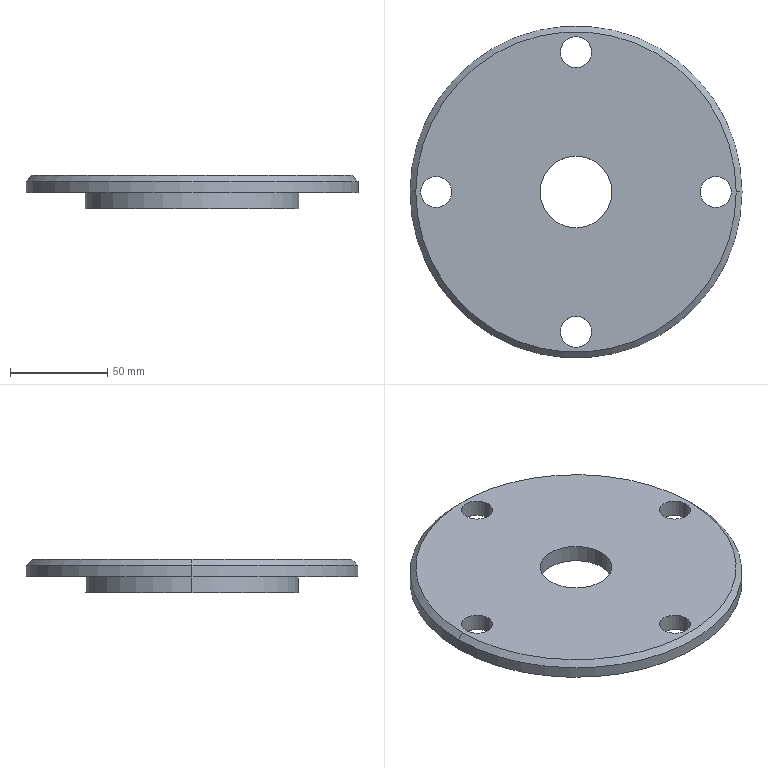Part | NX | features BREP 1 | 1 solid | 22 faces | box 171 x 171 x 17 mm | volume 205475 mm3 | cylinder 14 | cone 4 | plane 4 | commonest cylinder face diameters 16 x8 37 x2 110 x2 171 x2
STEP:
#1=CARTESIAN_POINT('',(-64.,0.,-9.));
#2=VERTEX_POINT('',#1);
#3=CARTESIAN_POINT('',(-80.,0.,-9.));
#4=VERTEX_POINT('',#3);
#5=CARTESIAN_POINT('',(-72.,0.,-9.));
#6=DIRECTION('',(0.,0.,-1.));
#7=DIRECTION('',(1.,0.,0.));
#8=AXIS2_PLACEMENT_3D('',#5,#6,#7);
#9=CIRCLE('',#8,8.);
#10=EDGE_CURVE('',#2,#4,#9,.T.);
#11=ORIENTED_EDGE('',*,*,#10,.T.);
#12=CARTESIAN_POINT('',(-80.,0.,0.));
#13=VERTEX_POINT('',#12);
#14=CARTESIAN_POINT('',(-80.,0.,-17.001));
#15=DIRECTION('',(0.,0.,1.));
#16=VECTOR('',#15,1000.);
#17=LINE('',#14,#16);
#18=EDGE_CURVE('',#4,#13,#17,.T.);
#19=ORIENTED_EDGE('',*,*,#18,.T.);
#20=CARTESIAN_POINT('',(-64.,0.,0.));
#21=VERTEX_POINT('',#20);
#22=CARTESIAN_POINT('',(-72.,0.,0.));
#23=DIRECTION('',(0.,0.,1.));
#24=DIRECTION('',(1.,0.,0.));
#25=AXIS2_PLACEMENT_3D('',#22,#23,#24);
#26=CIRCLE('',#25,8.);
#27=EDGE_CURVE('',#13,#21,#26,.T.);
#28=ORIENTED_EDGE('',*,*,#27,.T.);
#29=CARTESIAN_POINT('',(-64.,0.,-17.001));
#30=DIRECTION('',(0.,0.,1.));
#31=VECTOR('',#30,1000.);
#32=LINE('',#29,#31);
#33=EDGE_CURVE('',#2,#21,#32,.T.);
#34=ORIENTED_EDGE('',*,*,#33,.F.);
#35=EDGE_LOOP('',(#11,#19,#28,#34));
#36=FACE_BOUND('',#35,.T.);
#37=CARTESIAN_POINT('',(-72.,0.,-17.001));
#38=DIRECTION('',(0.,0.,1.));
#39=DIRECTION('',(-1.,0.,0.));
#40=AXIS2_PLACEMENT_3D('',#37,#38,#39);
#41=CYLINDRICAL_SURFACE('',#40,8.);
#42=ADVANCED_FACE('',(#36),#41,.F.);
#43=CARTESIAN_POINT('',(8.,-72.,-9.));
#44=VERTEX_POINT('',#43);
#45=CARTESIAN_POINT('',(-8.,-72.,-9.));
#46=VERTEX_POINT('',#45);
#47=CARTESIAN_POINT('',(0.,-72.,-9.));
#48=DIRECTION('',(0.,0.,-1.));
#49=DIRECTION('',(1.,0.,0.));
#50=AXIS2_PLACEMENT_3D('',#47,#48,#49);
#51=CIRCLE('',#50,8.);
#52=EDGE_CURVE('',#44,#46,#51,.T.);
#53=ORIENTED_EDGE('',*,*,#52,.T.);
#54=CARTESIAN_POINT('',(-8.,-72.,0.));
#55=VERTEX_POINT('',#54);
#56=CARTESIAN_POINT('',(-8.,-72.,-17.001));
#57=DIRECTION('',(0.,0.,1.));
#58=VECTOR('',#57,1000.);
#59=LINE('',#56,#58);
#60=EDGE_CURVE('',#46,#55,#59,.T.);
#61=ORIENTED_EDGE('',*,*,#60,.T.);
#62=CARTESIAN_POINT('',(8.,-72.,0.));
#63=VERTEX_POINT('',#62);
#64=CARTESIAN_POINT('',(0.,-72.,0.));
#65=DIRECTION('',(0.,0.,1.));
#66=DIRECTION('',(1.,0.,0.));
#67=AXIS2_PLACEMENT_3D('',#64,#65,#66);
#68=CIRCLE('',#67,8.);
#69=EDGE_CURVE('',#55,#63,#68,.T.);
#70=ORIENTED_EDGE('',*,*,#69,.T.);
#71=CARTESIAN_POINT('',(8.,-72.,-17.001));
#72=DIRECTION('',(0.,0.,1.));
#73=VECTOR('',#72,1000.);
#74=LINE('',#71,#73);
#75=EDGE_CURVE('',#44,#63,#74,.T.);
#76=ORIENTED_EDGE('',*,*,#75,.F.);
#77=EDGE_LOOP('',(#53,#61,#70,#76));
#78=FACE_BOUND('',#77,.T.);
#79=CARTESIAN_POINT('',(0.,-72.,-17.001));
#80=DIRECTION('',(0.,0.,1.));
#81=DIRECTION('',(-1.,0.,0.));
#82=AXIS2_PLACEMENT_3D('',#79,#80,#81);
#83=CYLINDRICAL_SURFACE('',#82,8.);
#84=ADVANCED_FACE('',(#78),#83,.F.);
#85=CARTESIAN_POINT('',(80.,0.,-9.));
#86=VERTEX_POINT('',#85);
#87=CARTESIAN_POINT('',(64.,0.,-9.));
#88=VERTEX_POINT('',#87);
#89=CARTESIAN_POINT('',(72.,0.,-9.));
#90=DIRECTION('',(0.,0.,-1.));
#91=DIRECTION('',(1.,0.,0.));
#92=AXIS2_PLACEMENT_3D('',#89,#90,#91);
#93=CIRCLE('',#92,8.);
#94=EDGE_CURVE('',#86,#88,#93,.T.);
#95=ORIENTED_EDGE('',*,*,#94,.T.);
#96=CARTESIAN_POINT('',(64.,0.,0.));
#97=VERTEX_POINT('',#96);
#98=CARTESIAN_POINT('',(64.,0.,-17.001));
#99=DIRECTION('',(0.,0.,1.));
#100=VECTOR('',#99,1000.);
#101=LINE('',#98,#100);
#102=EDGE_CURVE('',#88,#97,#101,.T.);
#103=ORIENTED_EDGE('',*,*,#102,.T.);
#104=CARTESIAN_POINT('',(80.,0.,0.));
#105=VERTEX_POINT('',#104);
#106=CARTESIAN_POINT('',(72.,0.,0.));
#107=DIRECTION('',(0.,0.,1.));
#108=DIRECTION('',(1.,0.,0.));
#109=AXIS2_PLACEMENT_3D('',#106,#107,#108);
#110=CIRCLE('',#109,8.);
#111=EDGE_CURVE('',#97,#105,#110,.T.);
#112=ORIENTED_EDGE('',*,*,#111,.T.);
#113=CARTESIAN_POINT('',(80.,0.,-17.001));
#114=DIRECTION('',(0.,0.,1.));
#115=VECTOR('',#114,1000.);
#116=LINE('',#113,#115);
#117=EDGE_CURVE('',#86,#105,#116,.T.);
#118=ORIENTED_EDGE('',*,*,#117,.F.);
#119=EDGE_LOOP('',(#95,#103,#112,#118));
#120=FACE_BOUND('',#119,.T.);
#121=CARTESIAN_POINT('',(72.,0.,-17.001));
#122=DIRECTION('',(0.,0.,1.));
#123=DIRECTION('',(-1.,0.,0.));
#124=AXIS2_PLACEMENT_3D('',#121,#122,#123);
#125=CYLINDRICAL_SURFACE('',#124,8.);
#126=ADVANCED_FACE('',(#120),#125,.F.);
#127=CARTESIAN_POINT('',(8.,72.,-9.));
#128=VERTEX_POINT('',#127);
#129=CARTESIAN_POINT('',(-8.,72.,-9.));
#130=VERTEX_POINT('',#129);
#131=CARTESIAN_POINT('',(0.,72.,-9.));
#132=DIRECTION('',(0.,0.,-1.));
#133=DIRECTION('',(1.,0.,0.));
#134=AXIS2_PLACEMENT_3D('',#131,#132,#133);
#135=CIRCLE('',#134,8.);
#136=EDGE_CURVE('',#128,#130,#135,.T.);
#137=ORIENTED_EDGE('',*,*,#136,.T.);
#138=CARTESIAN_POINT('',(-8.,72.,0.));
#139=VERTEX_POINT('',#138);
#140=CARTESIAN_POINT('',(-8.,72.,-17.001));
#141=DIRECTION('',(0.,0.,1.));
#142=VECTOR('',#141,1000.);
#143=LINE('',#140,#142);
#144=EDGE_CURVE('',#130,#139,#143,.T.);
#145=ORIENTED_EDGE('',*,*,#144,.T.);
#146=CARTESIAN_POINT('',(8.,72.,0.));
#147=VERTEX_POINT('',#146);
#148=CARTESIAN_POINT('',(0.,72.,0.));
#149=DIRECTION('',(0.,0.,1.));
#150=DIRECTION('',(1.,0.,0.));
#151=AXIS2_PLACEMENT_3D('',#148,#149,#150);
#152=CIRCLE('',#151,8.);
#153=EDGE_CURVE('',#139,#147,#152,.T.);
#154=ORIENTED_EDGE('',*,*,#153,.T.);
#155=CARTESIAN_POINT('',(8.,72.,-17.001));
#156=DIRECTION('',(0.,0.,1.));
#157=VECTOR('',#156,1000.);
#158=LINE('',#155,#157);
#159=EDGE_CURVE('',#128,#147,#158,.T.);
#160=ORIENTED_EDGE('',*,*,#159,.F.);
#161=EDGE_LOOP('',(#137,#145,#154,#160));
#162=FACE_BOUND('',#161,.T.);
#163=CARTESIAN_POINT('',(0.,72.,-17.001));
#164=DIRECTION('',(0.,0.,1.));
#165=DIRECTION('',(-1.,0.,0.));
#166=AXIS2_PLACEMENT_3D('',#163,#164,#165);
#167=CYLINDRICAL_SURFACE('',#166,8.);
#168=ADVANCED_FACE('',(#162),#167,.F.);
#169=CARTESIAN_POINT('',(-46.,0.,-9.));
#170=VERTEX_POINT('',#169);
#171=CARTESIAN_POINT('',(46.,0.,-9.));
#172=VERTEX_POINT('',#171);
#173=CARTESIAN_POINT('',(0.,0.,-9.));
#174=DIRECTION('',(0.,0.,1.));
#175=DIRECTION('',(1.,0.,0.));
#176=AXIS2_PLACEMENT_3D('',#173,#174,#175);
#177=CIRCLE('',#176,46.);
#178=EDGE_CURVE('',#170,#172,#177,.T.);
#179=ORIENTED_EDGE('',*,*,#178,.T.);
#180=CARTESIAN_POINT('',(50.,0.,-17.));
#181=VERTEX_POINT('',#180);
#182=CARTESIAN_POINT('',(46.,0.,-9.));
#183=DIRECTION('',(0.4472,0.,-0.8944));
#184=VECTOR('',#183,1000.);
#185=LINE('',#182,#184);
#186=EDGE_CURVE('',#181,#172,#185,.F.);
#187=ORIENTED_EDGE('',*,*,#186,.F.);
#188=CARTESIAN_POINT('',(-50.,0.,-17.));
#189=VERTEX_POINT('',#188);
#190=CARTESIAN_POINT('',(0.,0.,-17.));
#191=DIRECTION('',(0.,0.,1.));
#192=DIRECTION('',(1.,0.,0.));
#193=AXIS2_PLACEMENT_3D('',#190,#191,#192);
#194=CIRCLE('',#193,50.);
#195=EDGE_CURVE('',#189,#181,#194,.T.);
#196=ORIENTED_EDGE('',*,*,#195,.F.);
#197=CARTESIAN_POINT('',(-46.,0.,-9.));
#198=DIRECTION('',(-0.4472,0.,-0.8944));
#199=VECTOR('',#198,1000.);
#200=LINE('',#197,#199);
#201=EDGE_CURVE('',#189,#170,#200,.F.);
#202=ORIENTED_EDGE('',*,*,#201,.T.);
#203=EDGE_LOOP('',(#179,#187,#196,#202));
#204=FACE_BOUND('',#203,.T.);
#205=CARTESIAN_POINT('',(0.,0.,-9.));
#206=DIRECTION('',(0.,0.,-1.));
#207=DIRECTION('',(1.,0.,0.));
#208=AXIS2_PLACEMENT_3D('',#205,#206,#207);
#209=CONICAL_SURFACE('',#208,46.,0.4636);
#210=ADVANCED_FACE('',(#204),#209,.F.);
#211=CARTESIAN_POINT('',(55.,0.,-17.));
#212=VERTEX_POINT('',#211);
#213=CARTESIAN_POINT('',(-55.,0.,-17.));
#214=VERTEX_POINT('',#213);
#215=CARTESIAN_POINT('',(0.,0.,-17.));
#216=DIRECTION('',(0.,0.,1.));
#217=DIRECTION('',(1.,0.,0.));
#218=AXIS2_PLACEMENT_3D('',#215,#216,#217);
#219=CIRCLE('',#218,55.);
#220=EDGE_CURVE('',#212,#214,#219,.T.);
#221=ORIENTED_EDGE('',*,*,#220,.T.);
#222=CARTESIAN_POINT('',(-55.,0.,-9.));
#223=VERTEX_POINT('',#222);
#224=CARTESIAN_POINT('',(-55.,0.,0.));
#225=DIRECTION('',(0.,0.,1.));
#226=VECTOR('',#225,1000.);
#227=LINE('',#224,#226);
#228=EDGE_CURVE('',#214,#223,#227,.T.);
#229=ORIENTED_EDGE('',*,*,#228,.T.);
#230=CARTESIAN_POINT('',(55.,0.,-9.));
#231=VERTEX_POINT('',#230);
#232=CARTESIAN_POINT('',(0.,0.,-9.));
#233=DIRECTION('',(0.,0.,1.));
#234=DIRECTION('',(1.,0.,0.));
#235=AXIS2_PLACEMENT_3D('',#232,#233,#234);
#236=CIRCLE('',#235,55.);
#237=EDGE_CURVE('',#231,#223,#236,.T.);
#238=ORIENTED_EDGE('',*,*,#237,.F.);
#239=CARTESIAN_POINT('',(55.,0.,0.));
#240=DIRECTION('',(0.,0.,1.));
#241=VECTOR('',#240,1000.);
#242=LINE('',#239,#241);
#243=EDGE_CURVE('',#212,#231,#242,.T.);
#244=ORIENTED_EDGE('',*,*,#243,.F.);
#245=EDGE_LOOP('',(#221,#229,#238,#244));
#246=FACE_BOUND('',#245,.T.);
#247=CARTESIAN_POINT('',(0.,0.,0.));
#248=DIRECTION('',(0.,0.,1.));
#249=DIRECTION('',(-1.,0.,0.));
#250=AXIS2_PLACEMENT_3D('',#247,#248,#249);
#251=CYLINDRICAL_SURFACE('',#250,55.);
#252=ADVANCED_FACE('',(#246),#251,.T.);
#253=CARTESIAN_POINT('',(85.5,0.,-9.));
#254=VERTEX_POINT('',#253);
#255=CARTESIAN_POINT('',(-85.5,0.,-9.));
#256=VERTEX_POINT('',#255);
#257=CARTESIAN_POINT('',(0.,0.,-9.));
#258=DIRECTION('',(0.,0.,1.));
#259=DIRECTION('',(1.,0.,0.));
#260=AXIS2_PLACEMENT_3D('',#257,#258,#259);
#261=CIRCLE('',#260,85.5);
#262=EDGE_CURVE('',#254,#256,#261,.T.);
#263=ORIENTED_EDGE('',*,*,#262,.T.);
#264=CARTESIAN_POINT('',(-85.5,0.,-3.));
#265=VERTEX_POINT('',#264);
#266=CARTESIAN_POINT('',(-85.5,0.,0.));
#267=DIRECTION('',(0.,0.,1.));
#268=VECTOR('',#267,1000.);
#269=LINE('',#266,#268);
#270=EDGE_CURVE('',#256,#265,#269,.T.);
#271=ORIENTED_EDGE('',*,*,#270,.T.);
#272=CARTESIAN_POINT('',(85.5,0.,-3.));
#273=VERTEX_POINT('',#272);
#274=CARTESIAN_POINT('',(0.,0.,-3.));
#275=DIRECTION('',(0.,0.,1.));
#276=DIRECTION('',(1.,0.,0.));
#277=AXIS2_PLACEMENT_3D('',#274,#275,#276);
#278=CIRCLE('',#277,85.5);
#279=EDGE_CURVE('',#273,#265,#278,.T.);
#280=ORIENTED_EDGE('',*,*,#279,.F.);
#281=CARTESIAN_POINT('',(85.5,0.,0.));
#282=DIRECTION('',(0.,0.,1.));
#283=VECTOR('',#282,1000.);
#284=LINE('',#281,#283);
#285=EDGE_CURVE('',#254,#273,#284,.T.);
#286=ORIENTED_EDGE('',*,*,#285,.F.);
#287=EDGE_LOOP('',(#263,#271,#280,#286));
#288=FACE_BOUND('',#287,.T.);
#289=CARTESIAN_POINT('',(0.,0.,0.));
#290=DIRECTION('',(0.,0.,1.));
#291=DIRECTION('',(-1.,0.,0.));
#292=AXIS2_PLACEMENT_3D('',#289,#290,#291);
#293=CYLINDRICAL_SURFACE('',#292,85.5);
#294=ADVANCED_FACE('',(#288),#293,.T.);
#295=CARTESIAN_POINT('',(82.5,0.,0.));
#296=VERTEX_POINT('',#295);
#297=CARTESIAN_POINT('',(-82.5,0.,0.));
#298=VERTEX_POINT('',#297);
#299=CARTESIAN_POINT('',(0.,0.,0.));
#300=DIRECTION('',(0.,0.,1.));
#301=DIRECTION('',(1.,0.,0.));
#302=AXIS2_PLACEMENT_3D('',#299,#300,#301);
#303=CIRCLE('',#302,82.5);
#304=EDGE_CURVE('',#296,#298,#303,.T.);
#305=ORIENTED_EDGE('',*,*,#304,.F.);
#306=CARTESIAN_POINT('',(85.5,0.,-3.));
#307=DIRECTION('',(0.7071,0.,-0.7071));
#308=VECTOR('',#307,1000.);
#309=LINE('',#306,#308);
#310=EDGE_CURVE('',#273,#296,#309,.F.);
#311=ORIENTED_EDGE('',*,*,#310,.F.);
#312=ORIENTED_EDGE('',*,*,#279,.T.);
#313=CARTESIAN_POINT('',(-85.5,0.,-3.));
#314=DIRECTION('',(-0.7071,0.,-0.7071));
#315=VECTOR('',#314,1000.);
#316=LINE('',#313,#315);
#317=EDGE_CURVE('',#265,#298,#316,.F.);
#318=ORIENTED_EDGE('',*,*,#317,.T.);
#319=EDGE_LOOP('',(#305,#311,#312,#318));
#320=FACE_BOUND('',#319,.T.);
#321=CARTESIAN_POINT('',(0.,0.,-3.));
#322=DIRECTION('',(0.,0.,-1.));
#323=DIRECTION('',(1.,0.,0.));
#324=AXIS2_PLACEMENT_3D('',#321,#322,#323);
#325=CONICAL_SURFACE('',#324,85.5,0.7854);
#326=ADVANCED_FACE('',(#320),#325,.T.);
#327=CARTESIAN_POINT('',(-18.5,0.,-9.));
#328=VERTEX_POINT('',#327);
#329=CARTESIAN_POINT('',(18.5,0.,-9.));
#330=VERTEX_POINT('',#329);
#331=CARTESIAN_POINT('',(0.,0.,-9.));
#332=DIRECTION('',(0.,0.,1.));
#333=DIRECTION('',(1.,0.,0.));
#334=AXIS2_PLACEMENT_3D('',#331,#332,#333);
#335=CIRCLE('',#334,18.5);
#336=EDGE_CURVE('',#328,#330,#335,.T.);
#337=ORIENTED_EDGE('',*,*,#336,.F.);
#338=CARTESIAN_POINT('',(-18.5,0.,0.));
#339=VERTEX_POINT('',#338);
#340=CARTESIAN_POINT('',(-18.5,0.,0.));
#341=DIRECTION('',(0.,0.,1.));
#342=VECTOR('',#341,1000.);
#343=LINE('',#340,#342);
#344=EDGE_CURVE('',#328,#339,#343,.T.);
#345=ORIENTED_EDGE('',*,*,#344,.T.);
#346=CARTESIAN_POINT('',(18.5,0.,0.));
#347=VERTEX_POINT('',#346);
#348=CARTESIAN_POINT('',(0.,0.,0.));
#349=DIRECTION('',(0.,0.,1.));
#350=DIRECTION('',(1.,0.,0.));
#351=AXIS2_PLACEMENT_3D('',#348,#349,#350);
#352=CIRCLE('',#351,18.5);
#353=EDGE_CURVE('',#339,#347,#352,.T.);
#354=ORIENTED_EDGE('',*,*,#353,.T.);
#355=CARTESIAN_POINT('',(18.5,0.,0.));
#356=DIRECTION('',(0.,0.,1.));
#357=VECTOR('',#356,1000.);
#358=LINE('',#355,#357);
#359=EDGE_CURVE('',#330,#347,#358,.T.);
#360=ORIENTED_EDGE('',*,*,#359,.F.);
#361=EDGE_LOOP('',(#337,#345,#354,#360));
#362=FACE_BOUND('',#361,.T.);
#363=CARTESIAN_POINT('',(0.,0.,0.));
#364=DIRECTION('',(0.,0.,1.));
#365=DIRECTION('',(-1.,0.,0.));
#366=AXIS2_PLACEMENT_3D('',#363,#364,#365);
#367=CYLINDRICAL_SURFACE('',#366,18.5);
#368=ADVANCED_FACE('',(#362),#367,.F.);
#369=ORIENTED_EDGE('',*,*,#344,.F.);
#370=CARTESIAN_POINT('',(0.,0.,-9.));
#371=DIRECTION('',(0.,0.,1.));
#372=DIRECTION('',(1.,0.,0.));
#373=AXIS2_PLACEMENT_3D('',#370,#371,#372);
#374=CIRCLE('',#373,18.5);
#375=EDGE_CURVE('',#330,#328,#374,.T.);
#376=ORIENTED_EDGE('',*,*,#375,.F.);
#377=ORIENTED_EDGE('',*,*,#359,.T.);
#378=CARTESIAN_POINT('',(0.,0.,0.));
#379=DIRECTION('',(0.,0.,1.));
#380=DIRECTION('',(1.,0.,0.));
#381=AXIS2_PLACEMENT_3D('',#378,#379,#380);
#382=CIRCLE('',#381,18.5);
#383=EDGE_CURVE('',#347,#339,#382,.T.);
#384=ORIENTED_EDGE('',*,*,#383,.T.);
#385=EDGE_LOOP('',(#369,#376,#377,#384));
#386=FACE_BOUND('',#385,.T.);
#387=CARTESIAN_POINT('',(0.,0.,0.));
#388=DIRECTION('',(0.,0.,1.));
#389=DIRECTION('',(-1.,0.,0.));
#390=AXIS2_PLACEMENT_3D('',#387,#388,#389);
#391=CYLINDRICAL_SURFACE('',#390,18.5);
#392=ADVANCED_FACE('',(#386),#391,.F.);
#393=CARTESIAN_POINT('',(0.,0.,0.));
#394=DIRECTION('',(0.,0.,1.));
#395=DIRECTION('',(1.,0.,0.));
#396=AXIS2_PLACEMENT_3D('',#393,#394,#395);
#397=CIRCLE('',#396,82.5);
#398=EDGE_CURVE('',#298,#296,#397,.T.);
#399=ORIENTED_EDGE('',*,*,#398,.T.);
#400=ORIENTED_EDGE('',*,*,#304,.T.);
#401=EDGE_LOOP('',(#399,#400));
#402=FACE_BOUND('',#401,.T.);
#403=CARTESIAN_POINT('',(-72.,0.,0.));
#404=DIRECTION('',(0.,0.,1.));
#405=DIRECTION('',(1.,0.,0.));
#406=AXIS2_PLACEMENT_3D('',#403,#404,#405);
#407=CIRCLE('',#406,8.);
#408=EDGE_CURVE('',#21,#13,#407,.T.);
#409=ORIENTED_EDGE('',*,*,#408,.F.);
#410=ORIENTED_EDGE('',*,*,#27,.F.);
#411=EDGE_LOOP('',(#409,#410));
#412=FACE_BOUND('',#411,.T.);
#413=CARTESIAN_POINT('',(0.,-72.,0.));
#414=DIRECTION('',(0.,0.,1.));
#415=DIRECTION('',(1.,0.,0.));
#416=AXIS2_PLACEMENT_3D('',#413,#414,#415);
#417=CIRCLE('',#416,8.);
#418=EDGE_CURVE('',#63,#55,#417,.T.);
#419=ORIENTED_EDGE('',*,*,#418,.F.);
#420=ORIENTED_EDGE('',*,*,#69,.F.);
#421=EDGE_LOOP('',(#419,#420));
#422=FACE_BOUND('',#421,.T.);
#423=CARTESIAN_POINT('',(72.,0.,0.));
#424=DIRECTION('',(0.,0.,1.));
#425=DIRECTION('',(1.,0.,0.));
#426=AXIS2_PLACEMENT_3D('',#423,#424,#425);
#427=CIRCLE('',#426,8.);
#428=EDGE_CURVE('',#105,#97,#427,.T.);
#429=ORIENTED_EDGE('',*,*,#428,.F.);
#430=ORIENTED_EDGE('',*,*,#111,.F.);
#431=EDGE_LOOP('',(#429,#430));
#432=FACE_BOUND('',#431,.T.);
#433=CARTESIAN_POINT('',(0.,72.,0.));
#434=DIRECTION('',(0.,0.,1.));
#435=DIRECTION('',(1.,0.,0.));
#436=AXIS2_PLACEMENT_3D('',#433,#434,#435);
#437=CIRCLE('',#436,8.);
#438=EDGE_CURVE('',#147,#139,#437,.T.);
#439=ORIENTED_EDGE('',*,*,#438,.F.);
#440=ORIENTED_EDGE('',*,*,#153,.F.);
#441=EDGE_LOOP('',(#439,#440));
#442=FACE_BOUND('',#441,.T.);
#443=ORIENTED_EDGE('',*,*,#383,.F.);
#444=ORIENTED_EDGE('',*,*,#353,.F.);
#445=EDGE_LOOP('',(#443,#444));
#446=FACE_BOUND('',#445,.T.);
#447=CARTESIAN_POINT('',(0.,18.5,0.));
#448=DIRECTION('',(0.,0.,-1.));
#449=DIRECTION('',(1.,0.,0.));
#450=AXIS2_PLACEMENT_3D('',#447,#448,#449);
#451=PLANE('',#450);
#452=ADVANCED_FACE('',(#402,#412,#422,#432,#442,#446),#451,.F.);
#453=ORIENTED_EDGE('',*,*,#310,.T.);
#454=ORIENTED_EDGE('',*,*,#398,.F.);
#455=ORIENTED_EDGE('',*,*,#317,.F.);
#456=CARTESIAN_POINT('',(0.,0.,-3.));
#457=DIRECTION('',(0.,0.,1.));
#458=DIRECTION('',(1.,0.,0.));
#459=AXIS2_PLACEMENT_3D('',#456,#457,#458);
#460=CIRCLE('',#459,85.5);
#461=EDGE_CURVE('',#265,#273,#460,.T.);
#462=ORIENTED_EDGE('',*,*,#461,.T.);
#463=EDGE_LOOP('',(#453,#454,#455,#462));
#464=FACE_BOUND('',#463,.T.);
#465=CARTESIAN_POINT('',(0.,0.,-3.));
#466=DIRECTION('',(0.,0.,-1.));
#467=DIRECTION('',(1.,0.,0.));
#468=AXIS2_PLACEMENT_3D('',#465,#466,#467);
#469=CONICAL_SURFACE('',#468,85.5,0.7854);
#470=ADVANCED_FACE('',(#464),#469,.T.);
#471=ORIENTED_EDGE('',*,*,#270,.F.);
#472=CARTESIAN_POINT('',(0.,0.,-9.));
#473=DIRECTION('',(0.,0.,1.));
#474=DIRECTION('',(1.,0.,0.));
#475=AXIS2_PLACEMENT_3D('',#472,#473,#474);
#476=CIRCLE('',#475,85.5);
#477=EDGE_CURVE('',#256,#254,#476,.T.);
#478=ORIENTED_EDGE('',*,*,#477,.T.);
#479=ORIENTED_EDGE('',*,*,#285,.T.);
#480=ORIENTED_EDGE('',*,*,#461,.F.);
#481=EDGE_LOOP('',(#471,#478,#479,#480));
#482=FACE_BOUND('',#481,.T.);
#483=CARTESIAN_POINT('',(0.,0.,0.));
#484=DIRECTION('',(0.,0.,1.));
#485=DIRECTION('',(-1.,0.,0.));
#486=AXIS2_PLACEMENT_3D('',#483,#484,#485);
#487=CYLINDRICAL_SURFACE('',#486,85.5);
#488=ADVANCED_FACE('',(#482),#487,.T.);
#489=ORIENTED_EDGE('',*,*,#262,.F.);
#490=ORIENTED_EDGE('',*,*,#477,.F.);
#491=EDGE_LOOP('',(#489,#490));
#492=FACE_BOUND('',#491,.T.);
#493=ORIENTED_EDGE('',*,*,#10,.F.);
#494=CARTESIAN_POINT('',(-72.,0.,-9.));
#495=DIRECTION('',(0.,0.,-1.));
#496=DIRECTION('',(1.,0.,0.));
#497=AXIS2_PLACEMENT_3D('',#494,#495,#496);
#498=CIRCLE('',#497,8.);
#499=EDGE_CURVE('',#4,#2,#498,.T.);
#500=ORIENTED_EDGE('',*,*,#499,.F.);
#501=EDGE_LOOP('',(#493,#500));
#502=FACE_BOUND('',#501,.T.);
#503=ORIENTED_EDGE('',*,*,#52,.F.);
#504=CARTESIAN_POINT('',(0.,-72.,-9.));
#505=DIRECTION('',(0.,0.,-1.));
#506=DIRECTION('',(1.,0.,0.));
#507=AXIS2_PLACEMENT_3D('',#504,#505,#506);
#508=CIRCLE('',#507,8.);
#509=EDGE_CURVE('',#46,#44,#508,.T.);
#510=ORIENTED_EDGE('',*,*,#509,.F.);
#511=EDGE_LOOP('',(#503,#510));
#512=FACE_BOUND('',#511,.T.);
#513=ORIENTED_EDGE('',*,*,#94,.F.);
#514=CARTESIAN_POINT('',(72.,0.,-9.));
#515=DIRECTION('',(0.,0.,-1.));
#516=DIRECTION('',(1.,0.,0.));
#517=AXIS2_PLACEMENT_3D('',#514,#515,#516);
#518=CIRCLE('',#517,8.);
#519=EDGE_CURVE('',#88,#86,#518,.T.);
#520=ORIENTED_EDGE('',*,*,#519,.F.);
#521=EDGE_LOOP('',(#513,#520));
#522=FACE_BOUND('',#521,.T.);
#523=ORIENTED_EDGE('',*,*,#136,.F.);
#524=CARTESIAN_POINT('',(0.,72.,-9.));
#525=DIRECTION('',(0.,0.,-1.));
#526=DIRECTION('',(1.,0.,0.));
#527=AXIS2_PLACEMENT_3D('',#524,#525,#526);
#528=CIRCLE('',#527,8.);
#529=EDGE_CURVE('',#130,#128,#528,.T.);
#530=ORIENTED_EDGE('',*,*,#529,.F.);
#531=EDGE_LOOP('',(#523,#530));
#532=FACE_BOUND('',#531,.T.);
#533=ORIENTED_EDGE('',*,*,#237,.T.);
#534=CARTESIAN_POINT('',(0.,0.,-9.));
#535=DIRECTION('',(0.,0.,1.));
#536=DIRECTION('',(1.,0.,0.));
#537=AXIS2_PLACEMENT_3D('',#534,#535,#536);
#538=CIRCLE('',#537,55.);
#539=EDGE_CURVE('',#223,#231,#538,.T.);
#540=ORIENTED_EDGE('',*,*,#539,.T.);
#541=EDGE_LOOP('',(#533,#540));
#542=FACE_BOUND('',#541,.T.);
#543=CARTESIAN_POINT('',(0.,85.5,-9.));
#544=DIRECTION('',(0.,0.,1.));
#545=DIRECTION('',(0.,1.,0.));
#546=AXIS2_PLACEMENT_3D('',#543,#544,#545);
#547=PLANE('',#546);
#548=ADVANCED_FACE('',(#492,#502,#512,#522,#532,#542),#547,.F.);
#549=ORIENTED_EDGE('',*,*,#228,.F.);
#550=CARTESIAN_POINT('',(0.,0.,-17.));
#551=DIRECTION('',(0.,0.,1.));
#552=DIRECTION('',(1.,0.,0.));
#553=AXIS2_PLACEMENT_3D('',#550,#551,#552);
#554=CIRCLE('',#553,55.);
#555=EDGE_CURVE('',#214,#212,#554,.T.);
#556=ORIENTED_EDGE('',*,*,#555,.T.);
#557=ORIENTED_EDGE('',*,*,#243,.T.);
#558=ORIENTED_EDGE('',*,*,#539,.F.);
#559=EDGE_LOOP('',(#549,#556,#557,#558));
#560=FACE_BOUND('',#559,.T.);
#561=CARTESIAN_POINT('',(0.,0.,0.));
#562=DIRECTION('',(0.,0.,1.));
#563=DIRECTION('',(-1.,0.,0.));
#564=AXIS2_PLACEMENT_3D('',#561,#562,#563);
#565=CYLINDRICAL_SURFACE('',#564,55.);
#566=ADVANCED_FACE('',(#560),#565,.T.);
#567=ORIENTED_EDGE('',*,*,#220,.F.);
#568=ORIENTED_EDGE('',*,*,#555,.F.);
#569=EDGE_LOOP('',(#567,#568));
#570=FACE_BOUND('',#569,.T.);
#571=ORIENTED_EDGE('',*,*,#195,.T.);
#572=CARTESIAN_POINT('',(0.,0.,-17.));
#573=DIRECTION('',(0.,0.,1.));
#574=DIRECTION('',(1.,0.,0.));
#575=AXIS2_PLACEMENT_3D('',#572,#573,#574);
#576=CIRCLE('',#575,50.);
#577=EDGE_CURVE('',#181,#189,#576,.T.);
#578=ORIENTED_EDGE('',*,*,#577,.T.);
#579=EDGE_LOOP('',(#571,#578));
#580=FACE_BOUND('',#579,.T.);
#581=CARTESIAN_POINT('',(0.,55.,-17.));
#582=DIRECTION('',(0.,0.,1.));
#583=DIRECTION('',(0.,1.,0.));
#584=AXIS2_PLACEMENT_3D('',#581,#582,#583);
#585=PLANE('',#584);
#586=ADVANCED_FACE('',(#570,#580),#585,.F.);
#587=ORIENTED_EDGE('',*,*,#186,.T.);
#588=CARTESIAN_POINT('',(0.,0.,-9.));
#589=DIRECTION('',(0.,0.,1.));
#590=DIRECTION('',(1.,0.,0.));
#591=AXIS2_PLACEMENT_3D('',#588,#589,#590);
#592=CIRCLE('',#591,46.);
#593=EDGE_CURVE('',#172,#170,#592,.T.);
#594=ORIENTED_EDGE('',*,*,#593,.T.);
#595=ORIENTED_EDGE('',*,*,#201,.F.);
#596=ORIENTED_EDGE('',*,*,#577,.F.);
#597=EDGE_LOOP('',(#587,#594,#595,#596));
#598=FACE_BOUND('',#597,.T.);
#599=CARTESIAN_POINT('',(0.,0.,-9.));
#600=DIRECTION('',(0.,0.,-1.));
#601=DIRECTION('',(1.,0.,0.));
#602=AXIS2_PLACEMENT_3D('',#599,#600,#601);
#603=CONICAL_SURFACE('',#602,46.,0.4636);
#604=ADVANCED_FACE('',(#598),#603,.F.);
#605=ORIENTED_EDGE('',*,*,#178,.F.);
#606=ORIENTED_EDGE('',*,*,#593,.F.);
#607=EDGE_LOOP('',(#605,#606));
#608=FACE_BOUND('',#607,.T.);
#609=ORIENTED_EDGE('',*,*,#375,.T.);
#610=ORIENTED_EDGE('',*,*,#336,.T.);
#611=EDGE_LOOP('',(#609,#610));
#612=FACE_BOUND('',#611,.T.);
#613=CARTESIAN_POINT('',(0.,46.,-9.));
#614=DIRECTION('',(0.,0.,1.));
#615=DIRECTION('',(0.,1.,0.));
#616=AXIS2_PLACEMENT_3D('',#613,#614,#615);
#617=PLANE('',#616);
#618=ADVANCED_FACE('',(#608,#612),#617,.F.);
#619=ORIENTED_EDGE('',*,*,#144,.F.);
#620=ORIENTED_EDGE('',*,*,#529,.T.);
#621=ORIENTED_EDGE('',*,*,#159,.T.);
#622=ORIENTED_EDGE('',*,*,#438,.T.);
#623=EDGE_LOOP('',(#619,#620,#621,#622));
#624=FACE_BOUND('',#623,.T.);
#625=CARTESIAN_POINT('',(0.,72.,-17.001));
#626=DIRECTION('',(0.,0.,1.));
#627=DIRECTION('',(-1.,0.,0.));
#628=AXIS2_PLACEMENT_3D('',#625,#626,#627);
#629=CYLINDRICAL_SURFACE('',#628,8.);
#630=ADVANCED_FACE('',(#624),#629,.F.);
#631=ORIENTED_EDGE('',*,*,#102,.F.);
#632=ORIENTED_EDGE('',*,*,#519,.T.);
#633=ORIENTED_EDGE('',*,*,#117,.T.);
#634=ORIENTED_EDGE('',*,*,#428,.T.);
#635=EDGE_LOOP('',(#631,#632,#633,#634));
#636=FACE_BOUND('',#635,.T.);
#637=CARTESIAN_POINT('',(72.,0.,-17.001));
#638=DIRECTION('',(0.,0.,1.));
#639=DIRECTION('',(-1.,0.,0.));
#640=AXIS2_PLACEMENT_3D('',#637,#638,#639);
#641=CYLINDRICAL_SURFACE('',#640,8.);
#642=ADVANCED_FACE('',(#636),#641,.F.);
#643=ORIENTED_EDGE('',*,*,#60,.F.);
#644=ORIENTED_EDGE('',*,*,#509,.T.);
#645=ORIENTED_EDGE('',*,*,#75,.T.);
#646=ORIENTED_EDGE('',*,*,#418,.T.);
#647=EDGE_LOOP('',(#643,#644,#645,#646));
#648=FACE_BOUND('',#647,.T.);
#649=CARTESIAN_POINT('',(0.,-72.,-17.001));
#650=DIRECTION('',(0.,0.,1.));
#651=DIRECTION('',(-1.,0.,0.));
#652=AXIS2_PLACEMENT_3D('',#649,#650,#651);
#653=CYLINDRICAL_SURFACE('',#652,8.);
#654=ADVANCED_FACE('',(#648),#653,.F.);
#655=ORIENTED_EDGE('',*,*,#18,.F.);
#656=ORIENTED_EDGE('',*,*,#499,.T.);
#657=ORIENTED_EDGE('',*,*,#33,.T.);
#658=ORIENTED_EDGE('',*,*,#408,.T.);
#659=EDGE_LOOP('',(#655,#656,#657,#658));
#660=FACE_BOUND('',#659,.T.);
#661=CARTESIAN_POINT('',(-72.,0.,-17.001));
#662=DIRECTION('',(0.,0.,1.));
#663=DIRECTION('',(-1.,0.,0.));
#664=AXIS2_PLACEMENT_3D('',#661,#662,#663);
#665=CYLINDRICAL_SURFACE('',#664,8.);
#666=ADVANCED_FACE('',(#660),#665,.F.);
#667=CLOSED_SHELL('',(#42,#84,#126,#168,#210,#252,#294,#326,#368,#392,#452,#470,#488,#548,#566,#586,#604,#618,#630,#642,#654,#666));
#668=MANIFOLD_SOLID_BREP('',#667);
#669=(LENGTH_UNIT()NAMED_UNIT(*)SI_UNIT(.MILLI.,.METRE.));
#670=UNCERTAINTY_MEASURE_WITH_UNIT(LENGTH_MEASURE(0.00001),#669,'','');
#671=(NAMED_UNIT(*)PLANE_ANGLE_UNIT()SI_UNIT($,.RADIAN.));
#672=(NAMED_UNIT(*)SI_UNIT($,.STERADIAN.)SOLID_ANGLE_UNIT());
#673=(GEOMETRIC_REPRESENTATION_CONTEXT(3)GLOBAL_UNCERTAINTY_ASSIGNED_CONTEXT((#670))GLOBAL_UNIT_ASSIGNED_CONTEXT((#669,#671,#672))REPRESENTATION_CONTEXT('',''));
#674=ADVANCED_BREP_SHAPE_REPRESENTATION('',(#668),#673);